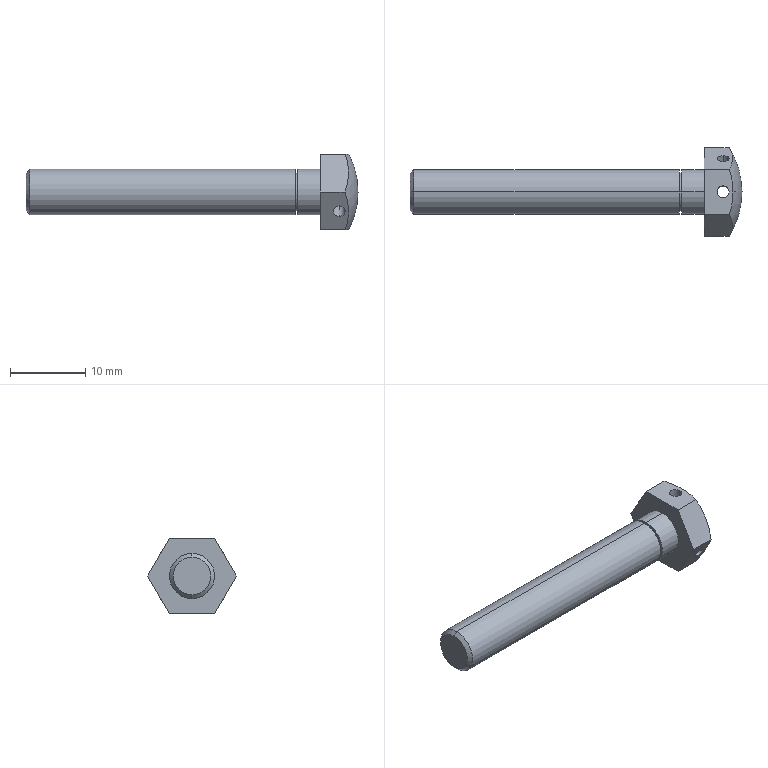Part | SolidWorks | features BaseBody 1 | 1 solid | 28 faces | box 44 x 11.759 x 10 mm | volume 1444 mm3 | cylinder 14 | plane 10 | cone 2 | sphere 2 | commonest cylinder face diameters 1.6 x8 6 x4 5 x2
STEP:
#1=CARTESIAN_POINT('',(392.6,48.19,57.147));
#2=VERTEX_POINT('',#1);
#3=CARTESIAN_POINT('',(392.6,48.99,55.761));
#4=VERTEX_POINT('',#3);
#5=CARTESIAN_POINT('',(392.6,48.59,56.454));
#6=DIRECTION('',(0.,0.866,0.5));
#7=DIRECTION('',(0.,0.5,-0.866));
#8=AXIS2_PLACEMENT_3D('',#5,#6,#7);
#9=CIRCLE('',#8,0.8);
#10=EDGE_CURVE('',#2,#4,#9,.T.);
#11=ORIENTED_EDGE('',*,*,#10,.F.);
#12=CARTESIAN_POINT('',(392.6,52.2,59.462));
#13=VERTEX_POINT('',#12);
#14=CARTESIAN_POINT('',(392.6,46.025,55.897));
#15=DIRECTION('',(0.,0.866,0.5));
#16=VECTOR('',#15,1000.);
#17=LINE('',#14,#16);
#18=EDGE_CURVE('',#2,#13,#17,.T.);
#19=ORIENTED_EDGE('',*,*,#18,.T.);
#20=CARTESIAN_POINT('',(393.4,53.,59.));
#21=VERTEX_POINT('',#20);
#22=CARTESIAN_POINT('',(393.4,53.,59.));
#23=CARTESIAN_POINT('',(393.4,52.531,59.271));
#24=CARTESIAN_POINT('',(393.069,52.2,59.462));
#25=CARTESIAN_POINT('',(392.6,52.2,59.462));
#26=(BOUNDED_CURVE()B_SPLINE_CURVE(3,(#22,#23,#24,#25),.UNSPECIFIED.,.F.,.F.)B_SPLINE_CURVE_WITH_KNOTS((4,4),(4.712,6.283),.UNSPECIFIED.)CURVE()GEOMETRIC_REPRESENTATION_ITEM()RATIONAL_B_SPLINE_CURVE((1.,0.8047,0.8047,1.))REPRESENTATION_ITEM(''));
#27=EDGE_CURVE('',#21,#13,#26,.T.);
#28=ORIENTED_EDGE('',*,*,#27,.F.);
#29=CARTESIAN_POINT('',(392.6,52.2,57.614));
#30=VERTEX_POINT('',#29);
#31=CARTESIAN_POINT('',(392.6,52.2,57.614));
#32=CARTESIAN_POINT('',(393.069,52.2,57.614));
#33=CARTESIAN_POINT('',(393.4,52.531,58.188));
#34=CARTESIAN_POINT('',(393.4,53.,59.));
#35=(BOUNDED_CURVE()B_SPLINE_CURVE(3,(#31,#32,#33,#34),.UNSPECIFIED.,.F.,.T.)B_SPLINE_CURVE_WITH_KNOTS((4,4),(3.142,4.712),.UNSPECIFIED.)CURVE()GEOMETRIC_REPRESENTATION_ITEM()RATIONAL_B_SPLINE_CURVE((1.,0.8047,0.8047,1.))REPRESENTATION_ITEM(''));
#36=EDGE_CURVE('',#30,#21,#35,.T.);
#37=ORIENTED_EDGE('',*,*,#36,.F.);
#38=CARTESIAN_POINT('',(392.6,46.825,54.511));
#39=DIRECTION('',(0.,0.866,0.5));
#40=VECTOR('',#39,1000.);
#41=LINE('',#38,#40);
#42=EDGE_CURVE('',#4,#30,#41,.T.);
#43=ORIENTED_EDGE('',*,*,#42,.F.);
#44=EDGE_LOOP('',(#11,#19,#28,#37,#43));
#45=FACE_OUTER_BOUND('',#44,.T.);
#46=CARTESIAN_POINT('',(392.6,46.425,55.204));
#47=DIRECTION('',(0.,0.866,0.5));
#48=DIRECTION('',(0.,0.5,-0.866));
#49=AXIS2_PLACEMENT_3D('',#46,#47,#48);
#50=CYLINDRICAL_SURFACE('',#49,0.8);
#51=ADVANCED_FACE('',(#45),#50,.F.);
#52=CARTESIAN_POINT('',(392.6,53.8,60.386));
#53=VERTEX_POINT('',#52);
#54=CARTESIAN_POINT('',(392.6,53.8,60.386));
#55=CARTESIAN_POINT('',(393.069,53.8,60.386));
#56=CARTESIAN_POINT('',(393.4,53.469,59.812));
#57=CARTESIAN_POINT('',(393.4,53.,59.));
#58=(BOUNDED_CURVE()B_SPLINE_CURVE(3,(#54,#55,#56,#57),.UNSPECIFIED.,.F.,.T.)B_SPLINE_CURVE_WITH_KNOTS((4,4),(0.,1.571),.UNSPECIFIED.)CURVE()GEOMETRIC_REPRESENTATION_ITEM()RATIONAL_B_SPLINE_CURVE((1.,0.8047,0.8047,1.))REPRESENTATION_ITEM(''));
#59=EDGE_CURVE('',#53,#21,#58,.T.);
#60=ORIENTED_EDGE('',*,*,#59,.F.);
#61=CARTESIAN_POINT('',(392.6,57.009,62.238));
#62=VERTEX_POINT('',#61);
#63=CARTESIAN_POINT('',(392.6,46.025,55.897));
#64=DIRECTION('',(0.,0.866,0.5));
#65=VECTOR('',#64,1000.);
#66=LINE('',#63,#65);
#67=EDGE_CURVE('',#53,#62,#66,.T.);
#68=ORIENTED_EDGE('',*,*,#67,.T.);
#69=CARTESIAN_POINT('',(392.6,57.809,60.853));
#70=VERTEX_POINT('',#69);
#71=CARTESIAN_POINT('',(392.6,57.409,61.546));
#72=DIRECTION('',(0.,0.866,0.5));
#73=DIRECTION('',(0.,0.5,-0.866));
#74=AXIS2_PLACEMENT_3D('',#71,#72,#73);
#75=CIRCLE('',#74,0.8);
#76=EDGE_CURVE('',#62,#70,#75,.T.);
#77=ORIENTED_EDGE('',*,*,#76,.T.);
#78=CARTESIAN_POINT('',(392.6,53.8,58.538));
#79=VERTEX_POINT('',#78);
#80=CARTESIAN_POINT('',(392.6,46.825,54.511));
#81=DIRECTION('',(0.,0.866,0.5));
#82=VECTOR('',#81,1000.);
#83=LINE('',#80,#82);
#84=EDGE_CURVE('',#79,#70,#83,.T.);
#85=ORIENTED_EDGE('',*,*,#84,.F.);
#86=CARTESIAN_POINT('',(393.4,53.,59.));
#87=CARTESIAN_POINT('',(393.4,53.469,58.729));
#88=CARTESIAN_POINT('',(393.069,53.8,58.538));
#89=CARTESIAN_POINT('',(392.6,53.8,58.538));
#90=(BOUNDED_CURVE()B_SPLINE_CURVE(3,(#86,#87,#88,#89),.UNSPECIFIED.,.F.,.F.)B_SPLINE_CURVE_WITH_KNOTS((4,4),(1.571,3.142),.UNSPECIFIED.)CURVE()GEOMETRIC_REPRESENTATION_ITEM()RATIONAL_B_SPLINE_CURVE((1.,0.8047,0.8047,1.))REPRESENTATION_ITEM(''));
#91=EDGE_CURVE('',#21,#79,#90,.T.);
#92=ORIENTED_EDGE('',*,*,#91,.F.);
#93=EDGE_LOOP('',(#60,#68,#77,#85,#92));
#94=FACE_OUTER_BOUND('',#93,.T.);
#95=CARTESIAN_POINT('',(392.6,46.425,55.204));
#96=DIRECTION('',(0.,0.866,0.5));
#97=DIRECTION('',(0.,0.5,-0.866));
#98=AXIS2_PLACEMENT_3D('',#95,#96,#97);
#99=CYLINDRICAL_SURFACE('',#98,0.8);
#100=ADVANCED_FACE('',(#94),#99,.F.);
#101=CARTESIAN_POINT('',(391.8,53.,54.));
#102=VERTEX_POINT('',#101);
#103=CARTESIAN_POINT('',(393.4,53.,54.));
#104=VERTEX_POINT('',#103);
#105=CARTESIAN_POINT('',(392.6,53.,54.));
#106=DIRECTION('',(0.,0.,1.));
#107=DIRECTION('',(1.,0.,0.));
#108=AXIS2_PLACEMENT_3D('',#105,#106,#107);
#109=CIRCLE('',#108,0.8);
#110=EDGE_CURVE('',#102,#104,#109,.T.);
#111=ORIENTED_EDGE('',*,*,#110,.F.);
#112=CARTESIAN_POINT('',(391.8,53.,59.));
#113=VERTEX_POINT('',#112);
#114=CARTESIAN_POINT('',(391.8,53.,54.));
#115=DIRECTION('',(0.,0.,1.));
#116=VECTOR('',#115,1000.);
#117=LINE('',#114,#116);
#118=EDGE_CURVE('',#102,#113,#117,.T.);
#119=ORIENTED_EDGE('',*,*,#118,.T.);
#120=CARTESIAN_POINT('',(391.8,53.,59.));
#121=CARTESIAN_POINT('',(391.8,52.531,58.188));
#122=CARTESIAN_POINT('',(392.131,52.2,57.614));
#123=CARTESIAN_POINT('',(392.6,52.2,57.614));
#124=(BOUNDED_CURVE()B_SPLINE_CURVE(3,(#120,#121,#122,#123),.UNSPECIFIED.,.F.,.F.)B_SPLINE_CURVE_WITH_KNOTS((4,4),(1.571,3.142),.UNSPECIFIED.)CURVE()GEOMETRIC_REPRESENTATION_ITEM()RATIONAL_B_SPLINE_CURVE((1.,0.8047,0.8047,1.))REPRESENTATION_ITEM(''));
#125=EDGE_CURVE('',#113,#30,#124,.T.);
#126=ORIENTED_EDGE('',*,*,#125,.T.);
#127=ORIENTED_EDGE('',*,*,#36,.T.);
#128=CARTESIAN_POINT('',(393.4,53.,54.));
#129=DIRECTION('',(0.,0.,1.));
#130=VECTOR('',#129,1000.);
#131=LINE('',#128,#130);
#132=EDGE_CURVE('',#104,#21,#131,.T.);
#133=ORIENTED_EDGE('',*,*,#132,.F.);
#134=EDGE_LOOP('',(#111,#119,#126,#127,#133));
#135=FACE_OUTER_BOUND('',#134,.T.);
#136=CARTESIAN_POINT('',(392.6,53.,54.));
#137=DIRECTION('',(0.,0.,1.));
#138=DIRECTION('',(1.,0.,0.));
#139=AXIS2_PLACEMENT_3D('',#136,#137,#138);
#140=CYLINDRICAL_SURFACE('',#139,0.8);
#141=ADVANCED_FACE('',(#135),#140,.F.);
#142=CARTESIAN_POINT('',(351.6,53.,56.));
#143=VERTEX_POINT('',#142);
#144=CARTESIAN_POINT('',(351.6,53.,62.));
#145=VERTEX_POINT('',#144);
#146=CARTESIAN_POINT('',(351.6,53.,59.));
#147=DIRECTION('',(1.,0.,0.));
#148=DIRECTION('',(0.,0.,1.));
#149=AXIS2_PLACEMENT_3D('',#146,#147,#148);
#150=CIRCLE('',#149,3.);
#151=EDGE_CURVE('',#143,#145,#150,.T.);
#152=ORIENTED_EDGE('',*,*,#151,.T.);
#153=CARTESIAN_POINT('',(386.8,53.,62.));
#154=VERTEX_POINT('',#153);
#155=CARTESIAN_POINT('',(351.1,53.,62.));
#156=DIRECTION('',(1.,0.,0.));
#157=VECTOR('',#156,1000.);
#158=LINE('',#155,#157);
#159=EDGE_CURVE('',#145,#154,#158,.T.);
#160=ORIENTED_EDGE('',*,*,#159,.T.);
#161=CARTESIAN_POINT('',(386.8,53.,56.));
#162=VERTEX_POINT('',#161);
#163=CARTESIAN_POINT('',(386.8,53.,59.));
#164=DIRECTION('',(1.,0.,0.));
#165=DIRECTION('',(0.,0.,-1.));
#166=AXIS2_PLACEMENT_3D('',#163,#164,#165);
#167=CIRCLE('',#166,3.);
#168=EDGE_CURVE('',#162,#154,#167,.T.);
#169=ORIENTED_EDGE('',*,*,#168,.F.);
#170=CARTESIAN_POINT('',(351.1,53.,56.));
#171=DIRECTION('',(1.,0.,0.));
#172=VECTOR('',#171,1000.);
#173=LINE('',#170,#172);
#174=EDGE_CURVE('',#143,#162,#173,.T.);
#175=ORIENTED_EDGE('',*,*,#174,.F.);
#176=EDGE_LOOP('',(#152,#160,#169,#175));
#177=FACE_OUTER_BOUND('',#176,.T.);
#178=CARTESIAN_POINT('',(351.1,53.,59.));
#179=DIRECTION('',(1.,0.,0.));
#180=DIRECTION('',(0.,0.,-1.));
#181=AXIS2_PLACEMENT_3D('',#178,#179,#180);
#182=CYLINDRICAL_SURFACE('',#181,3.);
#183=ADVANCED_FACE('',(#177),#182,.T.);
#184=CARTESIAN_POINT('',(351.1,53.,61.5));
#185=VERTEX_POINT('',#184);
#186=CARTESIAN_POINT('',(351.1,53.,56.5));
#187=VERTEX_POINT('',#186);
#188=CARTESIAN_POINT('',(351.1,53.,59.));
#189=DIRECTION('',(-1.,0.,0.));
#190=DIRECTION('',(0.,0.,1.));
#191=AXIS2_PLACEMENT_3D('',#188,#189,#190);
#192=CIRCLE('',#191,2.5);
#193=EDGE_CURVE('',#185,#187,#192,.T.);
#194=ORIENTED_EDGE('',*,*,#193,.F.);
#195=CARTESIAN_POINT('',(351.1,53.,61.5));
#196=DIRECTION('',(0.7071,0.,0.7071));
#197=VECTOR('',#196,1000.);
#198=LINE('',#195,#197);
#199=EDGE_CURVE('',#185,#145,#198,.T.);
#200=ORIENTED_EDGE('',*,*,#199,.T.);
#201=ORIENTED_EDGE('',*,*,#151,.F.);
#202=CARTESIAN_POINT('',(351.1,53.,56.5));
#203=DIRECTION('',(0.7071,0.,-0.7071));
#204=VECTOR('',#203,1000.);
#205=LINE('',#202,#204);
#206=EDGE_CURVE('',#187,#143,#205,.T.);
#207=ORIENTED_EDGE('',*,*,#206,.F.);
#208=EDGE_LOOP('',(#194,#200,#201,#207));
#209=FACE_OUTER_BOUND('',#208,.T.);
#210=CARTESIAN_POINT('',(351.1,53.,59.));
#211=DIRECTION('',(1.,0.,0.));
#212=DIRECTION('',(0.,0.,-1.));
#213=AXIS2_PLACEMENT_3D('',#210,#211,#212);
#214=CONICAL_SURFACE('',#213,2.5,0.7854);
#215=ADVANCED_FACE('',(#209),#214,.T.);
#216=CARTESIAN_POINT('',(386.8,53.,56.5));
#217=VERTEX_POINT('',#216);
#218=CARTESIAN_POINT('',(386.8,53.,61.5));
#219=VERTEX_POINT('',#218);
#220=CARTESIAN_POINT('',(386.8,53.,59.));
#221=DIRECTION('',(1.,0.,0.));
#222=DIRECTION('',(0.,0.,-1.));
#223=AXIS2_PLACEMENT_3D('',#220,#221,#222);
#224=CIRCLE('',#223,2.5);
#225=EDGE_CURVE('',#217,#219,#224,.T.);
#226=ORIENTED_EDGE('',*,*,#225,.T.);
#227=CARTESIAN_POINT('',(387.1,53.,61.5));
#228=VERTEX_POINT('',#227);
#229=CARTESIAN_POINT('',(396.833,53.,61.5));
#230=DIRECTION('',(1.,0.,0.));
#231=VECTOR('',#230,1000.);
#232=LINE('',#229,#231);
#233=EDGE_CURVE('',#219,#228,#232,.T.);
#234=ORIENTED_EDGE('',*,*,#233,.T.);
#235=CARTESIAN_POINT('',(387.1,53.,56.5));
#236=VERTEX_POINT('',#235);
#237=CARTESIAN_POINT('',(387.1,53.,59.));
#238=DIRECTION('',(1.,0.,0.));
#239=DIRECTION('',(0.,0.,-1.));
#240=AXIS2_PLACEMENT_3D('',#237,#238,#239);
#241=CIRCLE('',#240,2.5);
#242=EDGE_CURVE('',#236,#228,#241,.T.);
#243=ORIENTED_EDGE('',*,*,#242,.F.);
#244=CARTESIAN_POINT('',(396.833,53.,56.5));
#245=DIRECTION('',(1.,0.,0.));
#246=VECTOR('',#245,1000.);
#247=LINE('',#244,#246);
#248=EDGE_CURVE('',#217,#236,#247,.T.);
#249=ORIENTED_EDGE('',*,*,#248,.F.);
#250=EDGE_LOOP('',(#226,#234,#243,#249));
#251=FACE_OUTER_BOUND('',#250,.T.);
#252=CARTESIAN_POINT('',(396.833,53.,59.));
#253=DIRECTION('',(1.,0.,0.));
#254=DIRECTION('',(0.,0.,-1.));
#255=AXIS2_PLACEMENT_3D('',#252,#253,#254);
#256=CYLINDRICAL_SURFACE('',#255,2.5);
#257=ADVANCED_FACE('',(#251),#256,.T.);
#258=CARTESIAN_POINT('',(393.43,55.992,64.));
#259=VERTEX_POINT('',#258);
#260=CARTESIAN_POINT('',(393.898,53.,64.));
#261=VERTEX_POINT('',#260);
#262=CARTESIAN_POINT('',(384.1,53.,64.));
#263=DIRECTION('',(0.,0.,-1.));
#264=DIRECTION('',(-1.,0.,0.));
#265=AXIS2_PLACEMENT_3D('',#262,#263,#264);
#266=CIRCLE('',#265,9.798);
#267=EDGE_CURVE('',#259,#261,#266,.T.);
#268=ORIENTED_EDGE('',*,*,#267,.T.);
#269=CARTESIAN_POINT('',(395.1,53.,59.));
#270=VERTEX_POINT('',#269);
#271=CARTESIAN_POINT('',(384.1,53.,59.));
#272=DIRECTION('',(0.,1.,0.));
#273=DIRECTION('',(-1.,0.,0.));
#274=AXIS2_PLACEMENT_3D('',#271,#272,#273);
#275=CIRCLE('',#274,11.);
#276=EDGE_CURVE('',#261,#270,#275,.T.);
#277=ORIENTED_EDGE('',*,*,#276,.T.);
#278=CARTESIAN_POINT('',(393.898,53.,54.));
#279=VERTEX_POINT('',#278);
#280=CARTESIAN_POINT('',(384.1,53.,59.));
#281=DIRECTION('',(0.,-1.,0.));
#282=DIRECTION('',(1.,0.,0.));
#283=AXIS2_PLACEMENT_3D('',#280,#281,#282);
#284=CIRCLE('',#283,11.);
#285=EDGE_CURVE('',#279,#270,#284,.T.);
#286=ORIENTED_EDGE('',*,*,#285,.F.);
#287=CARTESIAN_POINT('',(393.43,55.992,54.));
#288=VERTEX_POINT('',#287);
#289=CARTESIAN_POINT('',(384.1,53.,54.));
#290=DIRECTION('',(0.,0.,1.));
#291=DIRECTION('',(1.,0.,0.));
#292=AXIS2_PLACEMENT_3D('',#289,#290,#291);
#293=CIRCLE('',#292,9.798);
#294=EDGE_CURVE('',#279,#288,#293,.T.);
#295=ORIENTED_EDGE('',*,*,#294,.T.);
#296=CARTESIAN_POINT('',(393.397,58.879,59.));
#297=VERTEX_POINT('',#296);
#298=CARTESIAN_POINT('',(384.1,57.409,56.454));
#299=DIRECTION('',(0.,-0.866,0.5));
#300=DIRECTION('',(0.,0.5,0.866));
#301=AXIS2_PLACEMENT_3D('',#298,#299,#300);
#302=CIRCLE('',#301,9.751);
#303=EDGE_CURVE('',#288,#297,#302,.T.);
#304=ORIENTED_EDGE('',*,*,#303,.T.);
#305=CARTESIAN_POINT('',(384.1,57.409,61.546));
#306=DIRECTION('',(0.,-0.866,-0.5));
#307=DIRECTION('',(0.,-0.5,0.866));
#308=AXIS2_PLACEMENT_3D('',#305,#306,#307);
#309=CIRCLE('',#308,9.751);
#310=EDGE_CURVE('',#297,#259,#309,.T.);
#311=ORIENTED_EDGE('',*,*,#310,.T.);
#312=EDGE_LOOP('',(#268,#277,#286,#295,#304,#311));
#313=FACE_OUTER_BOUND('',#312,.T.);
#314=CARTESIAN_POINT('',(384.1,53.,59.));
#315=DIRECTION('',(0.,1.,0.));
#316=DIRECTION('',(0.,0.,-1.));
#317=AXIS2_PLACEMENT_3D('',#314,#315,#316);
#318=SPHERICAL_SURFACE('',#317,11.);
#319=ADVANCED_FACE('',(#313),#318,.T.);
#320=CARTESIAN_POINT('',(387.1,53.,62.));
#321=VERTEX_POINT('',#320);
#322=CARTESIAN_POINT('',(387.1,53.,56.));
#323=VERTEX_POINT('',#322);
#324=CARTESIAN_POINT('',(387.1,53.,59.));
#325=DIRECTION('',(-1.,0.,0.));
#326=DIRECTION('',(0.,0.,1.));
#327=AXIS2_PLACEMENT_3D('',#324,#325,#326);
#328=CIRCLE('',#327,3.);
#329=EDGE_CURVE('',#321,#323,#328,.T.);
#330=ORIENTED_EDGE('',*,*,#329,.F.);
#331=CARTESIAN_POINT('',(390.1,53.,62.));
#332=VERTEX_POINT('',#331);
#333=CARTESIAN_POINT('',(351.1,53.,62.));
#334=DIRECTION('',(1.,0.,0.));
#335=VECTOR('',#334,1000.);
#336=LINE('',#333,#335);
#337=EDGE_CURVE('',#321,#332,#336,.T.);
#338=ORIENTED_EDGE('',*,*,#337,.T.);
#339=CARTESIAN_POINT('',(390.1,53.,56.));
#340=VERTEX_POINT('',#339);
#341=CARTESIAN_POINT('',(390.1,53.,59.));
#342=DIRECTION('',(-1.,0.,0.));
#343=DIRECTION('',(0.,0.,1.));
#344=AXIS2_PLACEMENT_3D('',#341,#342,#343);
#345=CIRCLE('',#344,3.);
#346=EDGE_CURVE('',#332,#340,#345,.T.);
#347=ORIENTED_EDGE('',*,*,#346,.T.);
#348=CARTESIAN_POINT('',(351.1,53.,56.));
#349=DIRECTION('',(1.,0.,0.));
#350=VECTOR('',#349,1000.);
#351=LINE('',#348,#350);
#352=EDGE_CURVE('',#323,#340,#351,.T.);
#353=ORIENTED_EDGE('',*,*,#352,.F.);
#354=EDGE_LOOP('',(#330,#338,#347,#353));
#355=FACE_OUTER_BOUND('',#354,.T.);
#356=CARTESIAN_POINT('',(351.1,53.,59.));
#357=DIRECTION('',(1.,0.,0.));
#358=DIRECTION('',(0.,0.,-1.));
#359=AXIS2_PLACEMENT_3D('',#356,#357,#358);
#360=CYLINDRICAL_SURFACE('',#359,3.);
#361=ADVANCED_FACE('',(#355),#360,.T.);
#362=ORIENTED_EDGE('',*,*,#27,.T.);
#363=CARTESIAN_POINT('',(392.6,52.2,59.462));
#364=CARTESIAN_POINT('',(392.131,52.2,59.462));
#365=CARTESIAN_POINT('',(391.8,52.531,59.271));
#366=CARTESIAN_POINT('',(391.8,53.,59.));
#367=(BOUNDED_CURVE()B_SPLINE_CURVE(3,(#363,#364,#365,#366),.UNSPECIFIED.,.F.,.T.)B_SPLINE_CURVE_WITH_KNOTS((4,4),(0.,1.571),.UNSPECIFIED.)CURVE()GEOMETRIC_REPRESENTATION_ITEM()RATIONAL_B_SPLINE_CURVE((1.,0.8047,0.8047,1.))REPRESENTATION_ITEM(''));
#368=EDGE_CURVE('',#13,#113,#367,.T.);
#369=ORIENTED_EDGE('',*,*,#368,.T.);
#370=CARTESIAN_POINT('',(391.8,53.,64.));
#371=VERTEX_POINT('',#370);
#372=CARTESIAN_POINT('',(391.8,53.,54.));
#373=DIRECTION('',(0.,0.,1.));
#374=VECTOR('',#373,1000.);
#375=LINE('',#372,#374);
#376=EDGE_CURVE('',#113,#371,#375,.T.);
#377=ORIENTED_EDGE('',*,*,#376,.T.);
#378=CARTESIAN_POINT('',(393.4,53.,64.));
#379=VERTEX_POINT('',#378);
#380=CARTESIAN_POINT('',(392.6,53.,64.));
#381=DIRECTION('',(0.,0.,1.));
#382=DIRECTION('',(1.,0.,0.));
#383=AXIS2_PLACEMENT_3D('',#380,#381,#382);
#384=CIRCLE('',#383,0.8);
#385=EDGE_CURVE('',#371,#379,#384,.T.);
#386=ORIENTED_EDGE('',*,*,#385,.T.);
#387=CARTESIAN_POINT('',(393.4,53.,54.));
#388=DIRECTION('',(0.,0.,1.));
#389=VECTOR('',#388,1000.);
#390=LINE('',#387,#389);
#391=EDGE_CURVE('',#21,#379,#390,.T.);
#392=ORIENTED_EDGE('',*,*,#391,.F.);
#393=EDGE_LOOP('',(#362,#369,#377,#386,#392));
#394=FACE_OUTER_BOUND('',#393,.T.);
#395=CARTESIAN_POINT('',(392.6,53.,54.));
#396=DIRECTION('',(0.,0.,1.));
#397=DIRECTION('',(1.,0.,0.));
#398=AXIS2_PLACEMENT_3D('',#395,#396,#397);
#399=CYLINDRICAL_SURFACE('',#398,0.8);
#400=ADVANCED_FACE('',(#394),#399,.F.);
#401=ORIENTED_EDGE('',*,*,#376,.F.);
#402=CARTESIAN_POINT('',(391.8,53.,59.));
#403=CARTESIAN_POINT('',(391.8,53.469,59.812));
#404=CARTESIAN_POINT('',(392.131,53.8,60.386));
#405=CARTESIAN_POINT('',(392.6,53.8,60.386));
#406=(BOUNDED_CURVE()B_SPLINE_CURVE(3,(#402,#403,#404,#405),.UNSPECIFIED.,.F.,.T.)B_SPLINE_CURVE_WITH_KNOTS((4,4),(4.712,6.283),.UNSPECIFIED.)CURVE()GEOMETRIC_REPRESENTATION_ITEM()RATIONAL_B_SPLINE_CURVE((1.,0.8047,0.8047,1.))REPRESENTATION_ITEM(''));
#407=EDGE_CURVE('',#113,#53,#406,.T.);
#408=ORIENTED_EDGE('',*,*,#407,.T.);
#409=ORIENTED_EDGE('',*,*,#59,.T.);
#410=ORIENTED_EDGE('',*,*,#391,.T.);
#411=CARTESIAN_POINT('',(392.6,53.,64.));
#412=DIRECTION('',(0.,0.,1.));
#413=DIRECTION('',(1.,0.,0.));
#414=AXIS2_PLACEMENT_3D('',#411,#412,#413);
#415=CIRCLE('',#414,0.8);
#416=EDGE_CURVE('',#379,#371,#415,.T.);
#417=ORIENTED_EDGE('',*,*,#416,.T.);
#418=EDGE_LOOP('',(#401,#408,#409,#410,#417));
#419=FACE_OUTER_BOUND('',#418,.T.);
#420=CARTESIAN_POINT('',(392.6,53.,54.));
#421=DIRECTION('',(0.,0.,1.));
#422=DIRECTION('',(1.,0.,0.));
#423=AXIS2_PLACEMENT_3D('',#420,#421,#422);
#424=CYLINDRICAL_SURFACE('',#423,0.8);
#425=ADVANCED_FACE('',(#419),#424,.F.);
#426=ORIENTED_EDGE('',*,*,#337,.F.);
#427=CARTESIAN_POINT('',(387.1,53.,59.));
#428=DIRECTION('',(-1.,0.,0.));
#429=DIRECTION('',(0.,0.,1.));
#430=AXIS2_PLACEMENT_3D('',#427,#428,#429);
#431=CIRCLE('',#430,3.);
#432=EDGE_CURVE('',#323,#321,#431,.T.);
#433=ORIENTED_EDGE('',*,*,#432,.F.);
#434=ORIENTED_EDGE('',*,*,#352,.T.);
#435=CARTESIAN_POINT('',(390.1,53.,59.));
#436=DIRECTION('',(-1.,0.,0.));
#437=DIRECTION('',(0.,0.,1.));
#438=AXIS2_PLACEMENT_3D('',#435,#436,#437);
#439=CIRCLE('',#438,3.);
#440=EDGE_CURVE('',#340,#332,#439,.T.);
#441=ORIENTED_EDGE('',*,*,#440,.T.);
#442=EDGE_LOOP('',(#426,#433,#434,#441));
#443=FACE_OUTER_BOUND('',#442,.T.);
#444=CARTESIAN_POINT('',(351.1,53.,59.));
#445=DIRECTION('',(1.,0.,0.));
#446=DIRECTION('',(0.,0.,-1.));
#447=AXIS2_PLACEMENT_3D('',#444,#445,#446);
#448=CYLINDRICAL_SURFACE('',#447,3.);
#449=ADVANCED_FACE('',(#443),#448,.T.);
#450=CARTESIAN_POINT('',(392.6,48.59,56.454));
#451=DIRECTION('',(0.,0.866,0.5));
#452=DIRECTION('',(0.,0.5,-0.866));
#453=AXIS2_PLACEMENT_3D('',#450,#451,#452);
#454=CIRCLE('',#453,0.8);
#455=EDGE_CURVE('',#4,#2,#454,.T.);
#456=ORIENTED_EDGE('',*,*,#455,.T.);
#457=ORIENTED_EDGE('',*,*,#10,.T.);
#458=EDGE_LOOP('',(#456,#457));
#459=FACE_BOUND('',#458,.T.);
#460=CARTESIAN_POINT('',(393.397,47.12,59.));
#461=VERTEX_POINT('',#460);
#462=CARTESIAN_POINT('',(393.43,50.007,54.));
#463=VERTEX_POINT('',#462);
#464=CARTESIAN_POINT('',(384.1,48.59,56.454));
#465=DIRECTION('',(0.,0.866,0.5));
#466=DIRECTION('',(0.,0.5,-0.866));
#467=AXIS2_PLACEMENT_3D('',#464,#465,#466);
#468=CIRCLE('',#467,9.75);
#469=EDGE_CURVE('',#461,#463,#468,.T.);
#470=ORIENTED_EDGE('',*,*,#469,.F.);
#471=CARTESIAN_POINT('',(390.1,47.12,59.));
#472=VERTEX_POINT('',#471);
#473=CARTESIAN_POINT('',(390.1,47.12,59.));
#474=DIRECTION('',(1.,0.,0.));
#475=VECTOR('',#474,1000.);
#476=LINE('',#473,#475);
#477=EDGE_CURVE('',#472,#461,#476,.T.);
#478=ORIENTED_EDGE('',*,*,#477,.F.);
#479=CARTESIAN_POINT('',(390.1,50.007,54.));
#480=VERTEX_POINT('',#479);
#481=CARTESIAN_POINT('',(390.1,47.12,59.));
#482=DIRECTION('',(0.,-0.5,0.866));
#483=VECTOR('',#482,1000.);
#484=LINE('',#481,#483);
#485=EDGE_CURVE('',#480,#472,#484,.T.);
#486=ORIENTED_EDGE('',*,*,#485,.F.);
#487=CARTESIAN_POINT('',(390.1,50.007,54.));
#488=DIRECTION('',(1.,0.,0.));
#489=VECTOR('',#488,1000.);
#490=LINE('',#487,#489);
#491=EDGE_CURVE('',#480,#463,#490,.T.);
#492=ORIENTED_EDGE('',*,*,#491,.T.);
#493=EDGE_LOOP('',(#470,#478,#486,#492));
#494=FACE_OUTER_BOUND('',#493,.T.);
#495=CARTESIAN_POINT('',(390.1,47.12,59.));
#496=DIRECTION('',(0.,0.866,0.5));
#497=DIRECTION('',(0.,0.5,-0.866));
#498=AXIS2_PLACEMENT_3D('',#495,#496,#497);
#499=PLANE('',#498);
#500=ADVANCED_FACE('',(#459,#494),#499,.F.);
#501=CARTESIAN_POINT('',(393.43,50.007,64.));
#502=VERTEX_POINT('',#501);
#503=CARTESIAN_POINT('',(384.1,48.59,61.546));
#504=DIRECTION('',(0.,0.866,-0.5));
#505=DIRECTION('',(0.,-0.5,-0.866));
#506=AXIS2_PLACEMENT_3D('',#503,#504,#505);
#507=CIRCLE('',#506,9.75);
#508=EDGE_CURVE('',#502,#461,#507,.T.);
#509=ORIENTED_EDGE('',*,*,#508,.F.);
#510=CARTESIAN_POINT('',(390.1,50.007,64.));
#511=VERTEX_POINT('',#510);
#512=CARTESIAN_POINT('',(390.1,50.007,64.));
#513=DIRECTION('',(1.,0.,0.));
#514=VECTOR('',#513,1000.);
#515=LINE('',#512,#514);
#516=EDGE_CURVE('',#511,#502,#515,.T.);
#517=ORIENTED_EDGE('',*,*,#516,.F.);
#518=CARTESIAN_POINT('',(390.1,47.12,59.));
#519=DIRECTION('',(0.,0.5,0.866));
#520=VECTOR('',#519,1000.);
#521=LINE('',#518,#520);
#522=EDGE_CURVE('',#472,#511,#521,.T.);
#523=ORIENTED_EDGE('',*,*,#522,.F.);
#524=ORIENTED_EDGE('',*,*,#477,.T.);
#525=EDGE_LOOP('',(#509,#517,#523,#524));
#526=FACE_OUTER_BOUND('',#525,.T.);
#527=CARTESIAN_POINT('',(390.1,47.12,59.));
#528=DIRECTION('',(0.,0.866,-0.5));
#529=DIRECTION('',(0.,-0.5,-0.866));
#530=AXIS2_PLACEMENT_3D('',#527,#528,#529);
#531=PLANE('',#530);
#532=ADVANCED_FACE('',(#526),#531,.F.);
#533=ORIENTED_EDGE('',*,*,#416,.F.);
#534=ORIENTED_EDGE('',*,*,#385,.F.);
#535=EDGE_LOOP('',(#533,#534));
#536=FACE_BOUND('',#535,.T.);
#537=ORIENTED_EDGE('',*,*,#267,.F.);
#538=CARTESIAN_POINT('',(390.1,55.992,64.));
#539=VERTEX_POINT('',#538);
#540=CARTESIAN_POINT('',(390.1,55.992,64.));
#541=DIRECTION('',(1.,0.,0.));
#542=VECTOR('',#541,1000.);
#543=LINE('',#540,#542);
#544=EDGE_CURVE('',#539,#259,#543,.T.);
#545=ORIENTED_EDGE('',*,*,#544,.F.);
#546=CARTESIAN_POINT('',(390.1,55.992,64.));
#547=DIRECTION('',(0.,1.,0.));
#548=VECTOR('',#547,1000.);
#549=LINE('',#546,#548);
#550=EDGE_CURVE('',#511,#539,#549,.T.);
#551=ORIENTED_EDGE('',*,*,#550,.F.);
#552=ORIENTED_EDGE('',*,*,#516,.T.);
#553=CARTESIAN_POINT('',(384.1,53.,64.));
#554=DIRECTION('',(0.,0.,-1.));
#555=DIRECTION('',(-1.,0.,0.));
#556=AXIS2_PLACEMENT_3D('',#553,#554,#555);
#557=CIRCLE('',#556,9.798);
#558=EDGE_CURVE('',#261,#502,#557,.T.);
#559=ORIENTED_EDGE('',*,*,#558,.F.);
#560=EDGE_LOOP('',(#537,#545,#551,#552,#559));
#561=FACE_OUTER_BOUND('',#560,.T.);
#562=CARTESIAN_POINT('',(390.1,55.992,64.));
#563=DIRECTION('',(0.,0.,-1.));
#564=DIRECTION('',(-1.,0.,0.));
#565=AXIS2_PLACEMENT_3D('',#562,#563,#564);
#566=PLANE('',#565);
#567=ADVANCED_FACE('',(#536,#561),#566,.F.);
#568=CARTESIAN_POINT('',(392.6,57.409,61.546));
#569=DIRECTION('',(0.,0.866,0.5));
#570=DIRECTION('',(0.,0.5,-0.866));
#571=AXIS2_PLACEMENT_3D('',#568,#569,#570);
#572=CIRCLE('',#571,0.8);
#573=EDGE_CURVE('',#70,#62,#572,.T.);
#574=ORIENTED_EDGE('',*,*,#573,.F.);
#575=ORIENTED_EDGE('',*,*,#76,.F.);
#576=EDGE_LOOP('',(#574,#575));
#577=FACE_BOUND('',#576,.T.);
#578=ORIENTED_EDGE('',*,*,#310,.F.);
#579=CARTESIAN_POINT('',(390.1,58.879,59.));
#580=VERTEX_POINT('',#579);
#581=CARTESIAN_POINT('',(390.1,58.879,59.));
#582=DIRECTION('',(1.,0.,0.));
#583=VECTOR('',#582,1000.);
#584=LINE('',#581,#583);
#585=EDGE_CURVE('',#580,#297,#584,.T.);
#586=ORIENTED_EDGE('',*,*,#585,.F.);
#587=CARTESIAN_POINT('',(390.1,58.879,59.));
#588=DIRECTION('',(0.,0.5,-0.866));
#589=VECTOR('',#588,1000.);
#590=LINE('',#587,#589);
#591=EDGE_CURVE('',#539,#580,#590,.T.);
#592=ORIENTED_EDGE('',*,*,#591,.F.);
#593=ORIENTED_EDGE('',*,*,#544,.T.);
#594=EDGE_LOOP('',(#578,#586,#592,#593));
#595=FACE_OUTER_BOUND('',#594,.T.);
#596=CARTESIAN_POINT('',(390.1,58.879,59.));
#597=DIRECTION('',(0.,-0.866,-0.5));
#598=DIRECTION('',(0.,-0.5,0.866));
#599=AXIS2_PLACEMENT_3D('',#596,#597,#598);
#600=PLANE('',#599);
#601=ADVANCED_FACE('',(#577,#595),#600,.F.);
#602=ORIENTED_EDGE('',*,*,#303,.F.);
#603=CARTESIAN_POINT('',(390.1,55.992,54.));
#604=VERTEX_POINT('',#603);
#605=CARTESIAN_POINT('',(390.1,55.992,54.));
#606=DIRECTION('',(1.,0.,0.));
#607=VECTOR('',#606,1000.);
#608=LINE('',#605,#607);
#609=EDGE_CURVE('',#604,#288,#608,.T.);
#610=ORIENTED_EDGE('',*,*,#609,.F.);
#611=CARTESIAN_POINT('',(390.1,58.879,59.));
#612=DIRECTION('',(0.,-0.5,-0.866));
#613=VECTOR('',#612,1000.);
#614=LINE('',#611,#613);
#615=EDGE_CURVE('',#580,#604,#614,.T.);
#616=ORIENTED_EDGE('',*,*,#615,.F.);
#617=ORIENTED_EDGE('',*,*,#585,.T.);
#618=EDGE_LOOP('',(#602,#610,#616,#617));
#619=FACE_OUTER_BOUND('',#618,.T.);
#620=CARTESIAN_POINT('',(390.1,58.879,59.));
#621=DIRECTION('',(0.,-0.866,0.5));
#622=DIRECTION('',(0.,0.5,0.866));
#623=AXIS2_PLACEMENT_3D('',#620,#621,#622);
#624=PLANE('',#623);
#625=ADVANCED_FACE('',(#619),#624,.F.);
#626=CARTESIAN_POINT('',(392.6,53.,54.));
#627=DIRECTION('',(0.,0.,1.));
#628=DIRECTION('',(1.,0.,0.));
#629=AXIS2_PLACEMENT_3D('',#626,#627,#628);
#630=CIRCLE('',#629,0.8);
#631=EDGE_CURVE('',#104,#102,#630,.T.);
#632=ORIENTED_EDGE('',*,*,#631,.T.);
#633=ORIENTED_EDGE('',*,*,#110,.T.);
#634=EDGE_LOOP('',(#632,#633));
#635=FACE_BOUND('',#634,.T.);
#636=CARTESIAN_POINT('',(384.1,53.,54.));
#637=DIRECTION('',(0.,0.,1.));
#638=DIRECTION('',(1.,0.,0.));
#639=AXIS2_PLACEMENT_3D('',#636,#637,#638);
#640=CIRCLE('',#639,9.798);
#641=EDGE_CURVE('',#463,#279,#640,.T.);
#642=ORIENTED_EDGE('',*,*,#641,.F.);
#643=ORIENTED_EDGE('',*,*,#491,.F.);
#644=CARTESIAN_POINT('',(390.1,55.992,54.));
#645=DIRECTION('',(0.,-1.,0.));
#646=VECTOR('',#645,1000.);
#647=LINE('',#644,#646);
#648=EDGE_CURVE('',#604,#480,#647,.T.);
#649=ORIENTED_EDGE('',*,*,#648,.F.);
#650=ORIENTED_EDGE('',*,*,#609,.T.);
#651=ORIENTED_EDGE('',*,*,#294,.F.);
#652=EDGE_LOOP('',(#642,#643,#649,#650,#651));
#653=FACE_OUTER_BOUND('',#652,.T.);
#654=CARTESIAN_POINT('',(390.1,55.992,54.));
#655=DIRECTION('',(0.,0.,1.));
#656=DIRECTION('',(1.,0.,0.));
#657=AXIS2_PLACEMENT_3D('',#654,#655,#656);
#658=PLANE('',#657);
#659=ADVANCED_FACE('',(#635,#653),#658,.F.);
#660=ORIENTED_EDGE('',*,*,#485,.T.);
#661=ORIENTED_EDGE('',*,*,#522,.T.);
#662=ORIENTED_EDGE('',*,*,#550,.T.);
#663=ORIENTED_EDGE('',*,*,#591,.T.);
#664=ORIENTED_EDGE('',*,*,#615,.T.);
#665=ORIENTED_EDGE('',*,*,#648,.T.);
#666=EDGE_LOOP('',(#660,#661,#662,#663,#664,#665));
#667=FACE_OUTER_BOUND('',#666,.T.);
#668=ORIENTED_EDGE('',*,*,#440,.F.);
#669=ORIENTED_EDGE('',*,*,#346,.F.);
#670=EDGE_LOOP('',(#668,#669));
#671=FACE_BOUND('',#670,.T.);
#672=CARTESIAN_POINT('',(390.1,50.007,54.));
#673=DIRECTION('',(-1.,0.,0.));
#674=DIRECTION('',(0.,0.,1.));
#675=AXIS2_PLACEMENT_3D('',#672,#673,#674);
#676=PLANE('',#675);
#677=ADVANCED_FACE('',(#667,#671),#676,.T.);
#678=ORIENTED_EDGE('',*,*,#276,.F.);
#679=ORIENTED_EDGE('',*,*,#558,.T.);
#680=ORIENTED_EDGE('',*,*,#508,.T.);
#681=ORIENTED_EDGE('',*,*,#469,.T.);
#682=ORIENTED_EDGE('',*,*,#641,.T.);
#683=ORIENTED_EDGE('',*,*,#285,.T.);
#684=EDGE_LOOP('',(#678,#679,#680,#681,#682,#683));
#685=FACE_OUTER_BOUND('',#684,.T.);
#686=CARTESIAN_POINT('',(384.1,53.,59.));
#687=DIRECTION('',(0.,1.,0.));
#688=DIRECTION('',(0.,0.,-1.));
#689=AXIS2_PLACEMENT_3D('',#686,#687,#688);
#690=SPHERICAL_SURFACE('',#689,11.);
#691=ADVANCED_FACE('',(#685),#690,.T.);
#692=ORIENTED_EDGE('',*,*,#225,.F.);
#693=CARTESIAN_POINT('',(386.8,53.,59.));
#694=DIRECTION('',(1.,0.,0.));
#695=DIRECTION('',(0.,0.,-1.));
#696=AXIS2_PLACEMENT_3D('',#693,#694,#695);
#697=CIRCLE('',#696,2.5);
#698=EDGE_CURVE('',#219,#217,#697,.T.);
#699=ORIENTED_EDGE('',*,*,#698,.F.);
#700=EDGE_LOOP('',(#692,#699));
#701=FACE_BOUND('',#700,.T.);
#702=ORIENTED_EDGE('',*,*,#168,.T.);
#703=CARTESIAN_POINT('',(386.8,53.,59.));
#704=DIRECTION('',(1.,0.,0.));
#705=DIRECTION('',(0.,0.,-1.));
#706=AXIS2_PLACEMENT_3D('',#703,#704,#705);
#707=CIRCLE('',#706,3.);
#708=EDGE_CURVE('',#154,#162,#707,.T.);
#709=ORIENTED_EDGE('',*,*,#708,.T.);
#710=EDGE_LOOP('',(#702,#709));
#711=FACE_OUTER_BOUND('',#710,.T.);
#712=CARTESIAN_POINT('',(386.8,53.,61.5));
#713=DIRECTION('',(1.,0.,0.));
#714=DIRECTION('',(0.,0.,-1.));
#715=AXIS2_PLACEMENT_3D('',#712,#713,#714);
#716=PLANE('',#715);
#717=ADVANCED_FACE('',(#701,#711),#716,.T.);
#718=ORIENTED_EDGE('',*,*,#242,.T.);
#719=CARTESIAN_POINT('',(387.1,53.,59.));
#720=DIRECTION('',(1.,0.,0.));
#721=DIRECTION('',(0.,0.,-1.));
#722=AXIS2_PLACEMENT_3D('',#719,#720,#721);
#723=CIRCLE('',#722,2.5);
#724=EDGE_CURVE('',#228,#236,#723,.T.);
#725=ORIENTED_EDGE('',*,*,#724,.T.);
#726=EDGE_LOOP('',(#718,#725));
#727=FACE_BOUND('',#726,.T.);
#728=ORIENTED_EDGE('',*,*,#432,.T.);
#729=ORIENTED_EDGE('',*,*,#329,.T.);
#730=EDGE_LOOP('',(#728,#729));
#731=FACE_OUTER_BOUND('',#730,.T.);
#732=CARTESIAN_POINT('',(387.1,53.,61.5));
#733=DIRECTION('',(-1.,0.,0.));
#734=DIRECTION('',(0.,0.,1.));
#735=AXIS2_PLACEMENT_3D('',#732,#733,#734);
#736=PLANE('',#735);
#737=ADVANCED_FACE('',(#727,#731),#736,.T.);
#738=ORIENTED_EDGE('',*,*,#233,.F.);
#739=ORIENTED_EDGE('',*,*,#698,.T.);
#740=ORIENTED_EDGE('',*,*,#248,.T.);
#741=ORIENTED_EDGE('',*,*,#724,.F.);
#742=EDGE_LOOP('',(#738,#739,#740,#741));
#743=FACE_OUTER_BOUND('',#742,.T.);
#744=CARTESIAN_POINT('',(396.833,53.,59.));
#745=DIRECTION('',(1.,0.,0.));
#746=DIRECTION('',(0.,0.,-1.));
#747=AXIS2_PLACEMENT_3D('',#744,#745,#746);
#748=CYLINDRICAL_SURFACE('',#747,2.5);
#749=ADVANCED_FACE('',(#743),#748,.T.);
#750=CARTESIAN_POINT('',(351.1,53.,59.));
#751=DIRECTION('',(-1.,0.,0.));
#752=DIRECTION('',(0.,0.,1.));
#753=AXIS2_PLACEMENT_3D('',#750,#751,#752);
#754=CIRCLE('',#753,2.5);
#755=EDGE_CURVE('',#187,#185,#754,.T.);
#756=ORIENTED_EDGE('',*,*,#755,.T.);
#757=ORIENTED_EDGE('',*,*,#193,.T.);
#758=EDGE_LOOP('',(#756,#757));
#759=FACE_OUTER_BOUND('',#758,.T.);
#760=CARTESIAN_POINT('',(351.1,53.,59.));
#761=DIRECTION('',(-1.,0.,0.));
#762=DIRECTION('',(0.,0.,1.));
#763=AXIS2_PLACEMENT_3D('',#760,#761,#762);
#764=PLANE('',#763);
#765=ADVANCED_FACE('',(#759),#764,.T.);
#766=ORIENTED_EDGE('',*,*,#199,.F.);
#767=ORIENTED_EDGE('',*,*,#755,.F.);
#768=ORIENTED_EDGE('',*,*,#206,.T.);
#769=CARTESIAN_POINT('',(351.6,53.,59.));
#770=DIRECTION('',(1.,0.,0.));
#771=DIRECTION('',(0.,0.,1.));
#772=AXIS2_PLACEMENT_3D('',#769,#770,#771);
#773=CIRCLE('',#772,3.);
#774=EDGE_CURVE('',#145,#143,#773,.T.);
#775=ORIENTED_EDGE('',*,*,#774,.F.);
#776=EDGE_LOOP('',(#766,#767,#768,#775));
#777=FACE_OUTER_BOUND('',#776,.T.);
#778=CARTESIAN_POINT('',(351.1,53.,59.));
#779=DIRECTION('',(1.,0.,0.));
#780=DIRECTION('',(0.,0.,-1.));
#781=AXIS2_PLACEMENT_3D('',#778,#779,#780);
#782=CONICAL_SURFACE('',#781,2.5,0.7854);
#783=ADVANCED_FACE('',(#777),#782,.T.);
#784=ORIENTED_EDGE('',*,*,#159,.F.);
#785=ORIENTED_EDGE('',*,*,#774,.T.);
#786=ORIENTED_EDGE('',*,*,#174,.T.);
#787=ORIENTED_EDGE('',*,*,#708,.F.);
#788=EDGE_LOOP('',(#784,#785,#786,#787));
#789=FACE_OUTER_BOUND('',#788,.T.);
#790=CARTESIAN_POINT('',(351.1,53.,59.));
#791=DIRECTION('',(1.,0.,0.));
#792=DIRECTION('',(0.,0.,-1.));
#793=AXIS2_PLACEMENT_3D('',#790,#791,#792);
#794=CYLINDRICAL_SURFACE('',#793,3.);
#795=ADVANCED_FACE('',(#789),#794,.T.);
#796=ORIENTED_EDGE('',*,*,#118,.F.);
#797=ORIENTED_EDGE('',*,*,#631,.F.);
#798=ORIENTED_EDGE('',*,*,#132,.T.);
#799=ORIENTED_EDGE('',*,*,#91,.T.);
#800=CARTESIAN_POINT('',(392.6,53.8,58.538));
#801=CARTESIAN_POINT('',(392.131,53.8,58.538));
#802=CARTESIAN_POINT('',(391.8,53.469,58.729));
#803=CARTESIAN_POINT('',(391.8,53.,59.));
#804=(BOUNDED_CURVE()B_SPLINE_CURVE(3,(#800,#801,#802,#803),.UNSPECIFIED.,.F.,.F.)B_SPLINE_CURVE_WITH_KNOTS((4,4),(3.142,4.712),.UNSPECIFIED.)CURVE()GEOMETRIC_REPRESENTATION_ITEM()RATIONAL_B_SPLINE_CURVE((1.,0.8047,0.8047,1.))REPRESENTATION_ITEM(''));
#805=EDGE_CURVE('',#79,#113,#804,.T.);
#806=ORIENTED_EDGE('',*,*,#805,.T.);
#807=EDGE_LOOP('',(#796,#797,#798,#799,#806));
#808=FACE_OUTER_BOUND('',#807,.T.);
#809=CARTESIAN_POINT('',(392.6,53.,54.));
#810=DIRECTION('',(0.,0.,1.));
#811=DIRECTION('',(1.,0.,0.));
#812=AXIS2_PLACEMENT_3D('',#809,#810,#811);
#813=CYLINDRICAL_SURFACE('',#812,0.8);
#814=ADVANCED_FACE('',(#808),#813,.F.);
#815=ORIENTED_EDGE('',*,*,#67,.F.);
#816=ORIENTED_EDGE('',*,*,#407,.F.);
#817=ORIENTED_EDGE('',*,*,#805,.F.);
#818=ORIENTED_EDGE('',*,*,#84,.T.);
#819=ORIENTED_EDGE('',*,*,#573,.T.);
#820=EDGE_LOOP('',(#815,#816,#817,#818,#819));
#821=FACE_OUTER_BOUND('',#820,.T.);
#822=CARTESIAN_POINT('',(392.6,46.425,55.204));
#823=DIRECTION('',(0.,0.866,0.5));
#824=DIRECTION('',(0.,0.5,-0.866));
#825=AXIS2_PLACEMENT_3D('',#822,#823,#824);
#826=CYLINDRICAL_SURFACE('',#825,0.8);
#827=ADVANCED_FACE('',(#821),#826,.F.);
#828=ORIENTED_EDGE('',*,*,#18,.F.);
#829=ORIENTED_EDGE('',*,*,#455,.F.);
#830=ORIENTED_EDGE('',*,*,#42,.T.);
#831=ORIENTED_EDGE('',*,*,#125,.F.);
#832=ORIENTED_EDGE('',*,*,#368,.F.);
#833=EDGE_LOOP('',(#828,#829,#830,#831,#832));
#834=FACE_OUTER_BOUND('',#833,.T.);
#835=CARTESIAN_POINT('',(392.6,46.425,55.204));
#836=DIRECTION('',(0.,0.866,0.5));
#837=DIRECTION('',(0.,0.5,-0.866));
#838=AXIS2_PLACEMENT_3D('',#835,#836,#837);
#839=CYLINDRICAL_SURFACE('',#838,0.8);
#840=ADVANCED_FACE('',(#834),#839,.F.);
#841=CLOSED_SHELL('',(#51,#100,#141,#183,#215,#257,#319,#361,#400,#425,#449,#500,#532,#567,#601,#625,#659,#677,#691,#717,#737,#749,#765,#783,#795,#814,#827,#840));
#842=MANIFOLD_SOLID_BREP('',#841);
#843=CARTESIAN_POINT('',(0.,0.,0.));
#844=DIRECTION('',(0.,0.,1.));
#845=DIRECTION('',(1.,0.,0.));
#846=AXIS2_PLACEMENT_3D('',#843,#844,#845);
#847=(LENGTH_UNIT()NAMED_UNIT(*)SI_UNIT(.MILLI.,.METRE.));
#848=UNCERTAINTY_MEASURE_WITH_UNIT(LENGTH_MEASURE(0.00001),#847,'','');
#849=(NAMED_UNIT(*)PLANE_ANGLE_UNIT()SI_UNIT($,.RADIAN.));
#850=(NAMED_UNIT(*)SI_UNIT($,.STERADIAN.)SOLID_ANGLE_UNIT());
#851=(GEOMETRIC_REPRESENTATION_CONTEXT(3)GLOBAL_UNCERTAINTY_ASSIGNED_CONTEXT((#848))GLOBAL_UNIT_ASSIGNED_CONTEXT((#847,#849,#850))REPRESENTATION_CONTEXT('',''));
#852=ADVANCED_BREP_SHAPE_REPRESENTATION('',(#842,#846),#851);